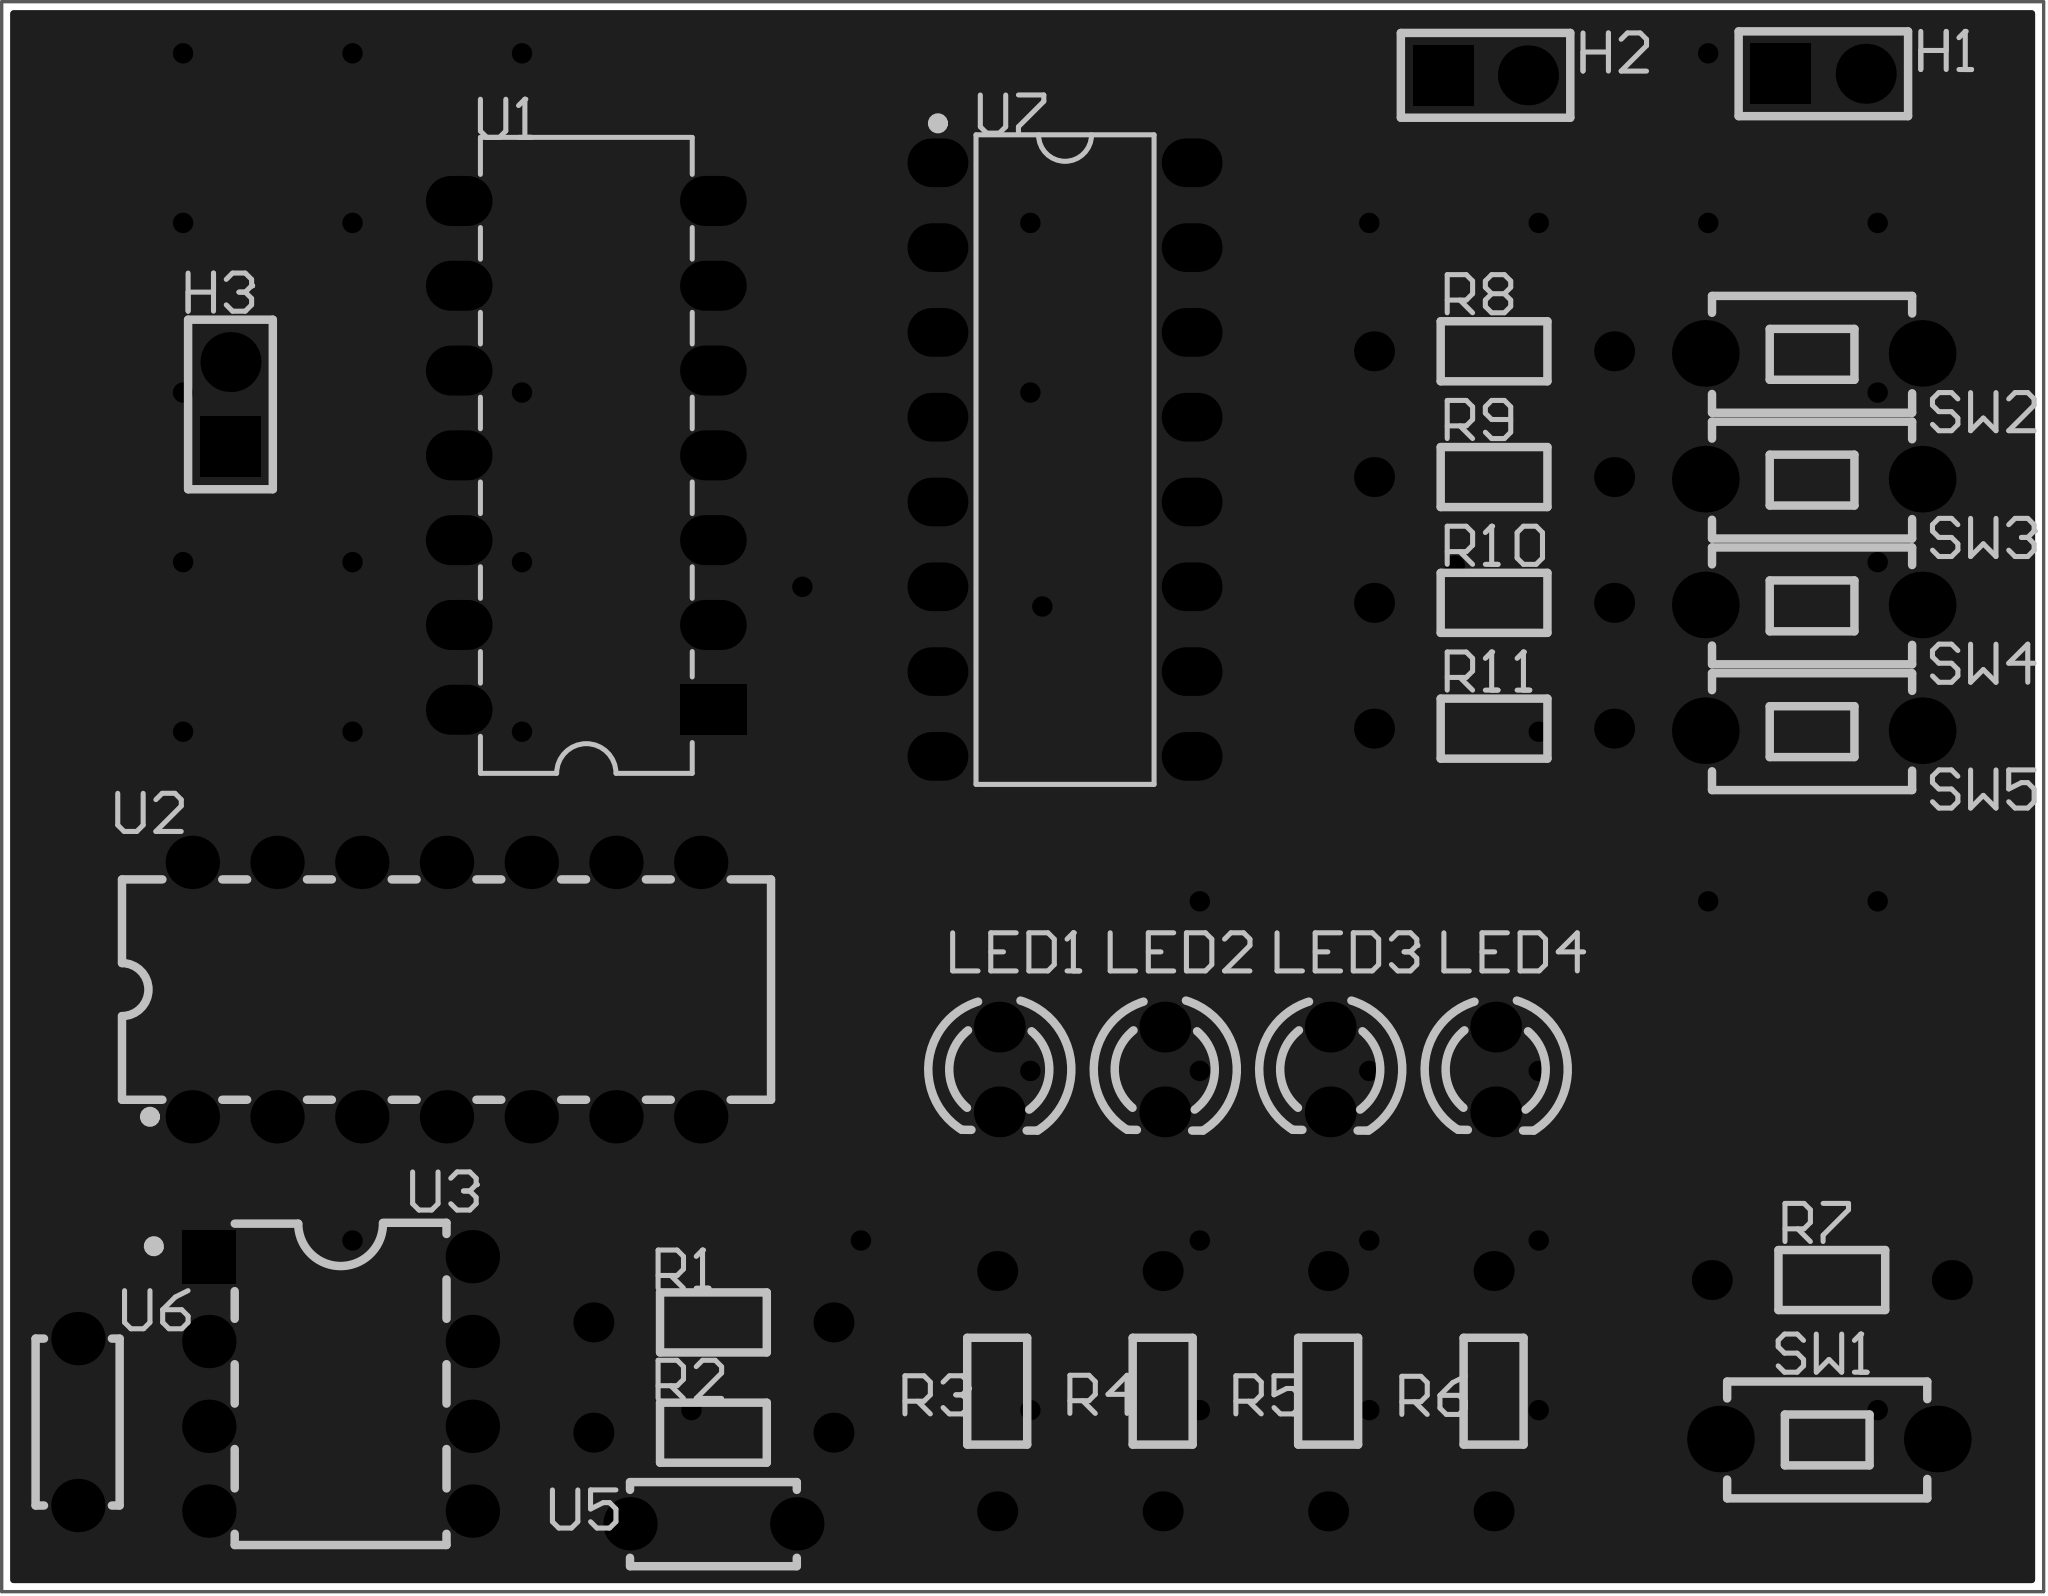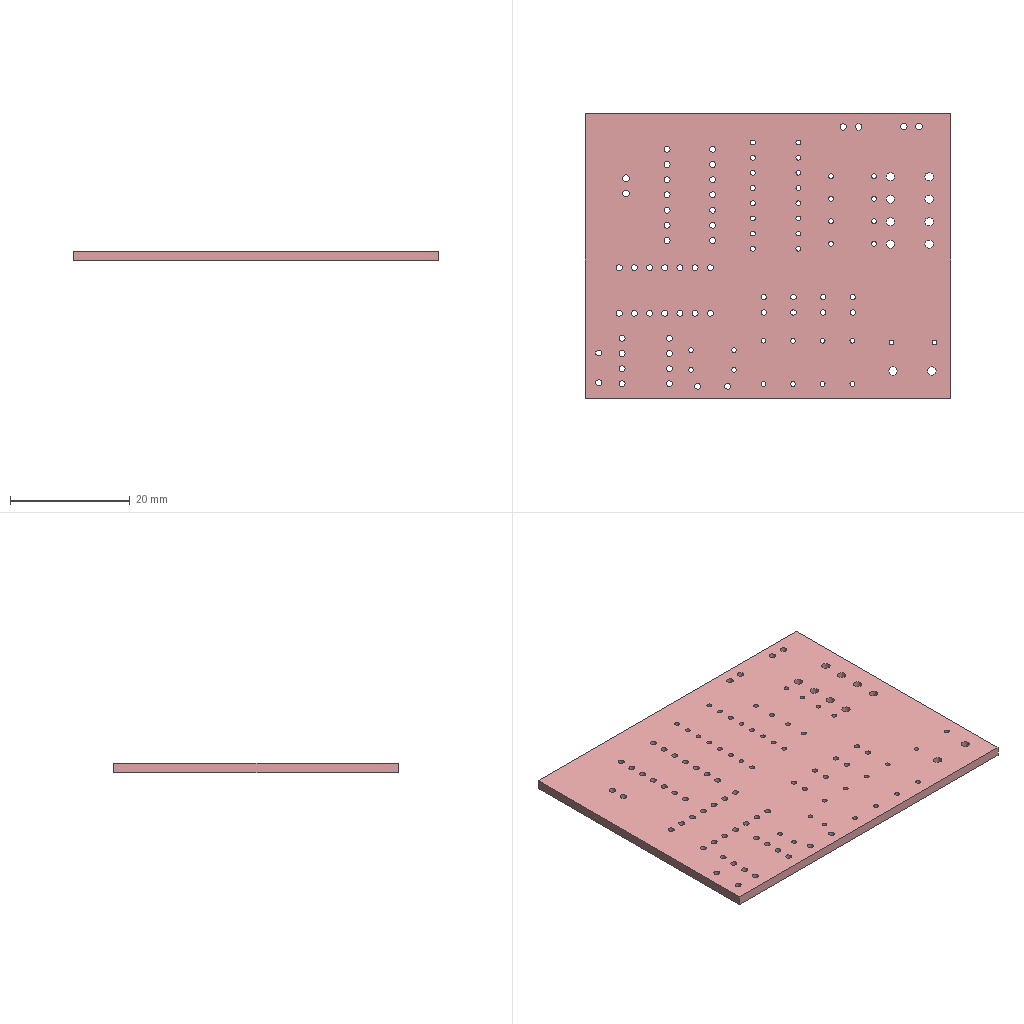Circuit board layout | Altium Designer | box 61.2 x 47.6 x 1.6 mm
Layer stack:
# Altium Designer layer stack of  (unit mm; dielectric type: 0 none, 1 core, 2 prepreg, 3 surface material)
index,name,kind,layer,copper_thickness_mm,dielectric_type,dielectric_thickness_mm,dielectric_material,dielectric_constant
0,Top Paste Mask Layer,other,,,,,,
1,Top Silkscreen Layer,other,,,,,,
2,Top Solder Mask Layer,dielectric,,,3,0.01,,3.3
3,Top Layer,copper,Top Layer,0.035,,,,
4,Dielectric1,dielectric,,,3,1.51,FR4,4.5
5,Bottom Layer,copper,Bottom Layer,0.035,,,,
6,Bottom Solder Mask Layer,dielectric,,,3,0.01,,3.3
7,Bottom Silkscreen Layer,other,,,,,,
8,Bottom Paste Mask Layer,other,,,,,,
# drill layer pairs: low layer,high layer
drill_pair,Top Layer,Bottom Layer
Part placement:
Designator,Comment,Layer,Footprint,Center-X(mm),Center-Y(mm),Rotation
H1,,TopLayer,HDR-TH_2P-P2.54-V-M-1,134.239,123.698,0
H2,,TopLayer,HDR-TH_2P-P2.54-V-M-1,124.113,123.651,0
H3,,TopLayer,HDR-TH_2P-P2.54-V-M-1,86.487,113.792,90
LED1,,TopLayer,LED_TH-3mm,109.535,93.873,270
LED2,,TopLayer,LED_TH-3mm,114.496,93.873,270
LED3,,TopLayer,LED_TH-3mm,119.456,93.873,270
LED4,,TopLayer,LED_TH-3mm,124.416,93.873,270
R1,4.3kΩ,TopLayer,Res_1/8W,100.965,86.296,0
R2,5.1kΩ,TopLayer,Res_1/8W,100.965,82.994,0
R3,220Ω,TopLayer,Res_1/8W,109.473,84.237,90
R4,220Ω,TopLayer,Res_1/8W,114.433,84.237,90
R5,220Ω,TopLayer,Res_1/8W,119.393,84.237,90
R6,220Ω,TopLayer,Res_1/8W,124.353,84.237,90
R7,10kΩ,TopLayer,Res_1/8W,134.493,87.566,0
R8,10kΩ,TopLayer,Res_1/8W,124.367,115.385,0
R9,10kΩ,TopLayer,Res_1/8W,124.367,111.618,0
R10,10kΩ,TopLayer,Res_1/8W,124.367,107.85,0
R11,10kΩ,TopLayer,Res_1/8W,124.367,104.082,0
SW1,,TopLayer,Key_TH_3.5x6x4.3,134.404,82.804,0
SW2,,TopLayer,Key_TH_3.5x6x4.3,133.95,115.322,0
SW3,,TopLayer,Key_TH_3.5x6x4.3,133.95,111.555,0
SW4,,TopLayer,Key_TH_3.5x6x4.3,133.95,107.787,0
SW5,,TopLayer,Key_TH_3.5x6x4.3,133.95,104.02,0
U1,SN74LS20N(XBLW),TopLayer,DIP-14_L19.0-W6.4-P2.54-LS7.6-BL,97.155,112.268,90
U2,SN74LS00NE4,TopLayer,PDIP-14_L19.3-W6.4-P2.54-LS7.9-BL,92.964,96.266,0
U3,LM555CM,TopLayer,PDIP-8_L9.6-W6.4-P2.54-LS7.9-BL-1,89.789,84.455,270
U5,10nF,TopLayer,CAP-TH_L5.0-W2.5-P5.00-D1.0,100.965,80.264,0
U6,100nF,TopLayer,CAP-TH_L5.0-W2.5-P5.00-D1.0,81.915,83.312,270
U7,SN74LS175N,TopLayer,DIP-16_L19.3-W6.4-P2.54-LS7.6-BL,111.506,112.141,270
Pad and via stacks:
# Altium Designer via and pad stacks of  (unit mm). Each distinct definition once, with the count of objects using it.
# via: kind,start_layer,end_layer,hole_mm,diameter_mm,mode(0 simple;1 top-mid-bottom;2 full stack),diameter_per_layer,count,example_net
# pad: kind,layer,hole_mm,hole_type(0 round;1 square;2 slot),plating,top_size,top_shape(1 round;2 rect;3 octagon;9 rounded rect),mid_size,bottom_size,mode,footprint,size_per_layer,count,example
pad,Multi-Layer,1.1,0,plated,1.8x1.8,1,1.8x1.8,1.8x1.8,0,HDR-TH_2P-P2.54-V-M-1,,3,H1.2
pad,Multi-Layer,1.1,0,plated,1.8x1.8,2,1.8x1.8,1.8x1.8,0,HDR-TH_2P-P2.54-V-M-1,,3,H1.1
pad,Multi-Layer,0.9144,0,plated,1.524x1.524,1,1.524x1.524,1.524x1.524,0,LED_TH-3mm,,8,LED1.1
pad,Multi-Layer,0.8001,0,plated,1.199x1.199,1,1.199x1.199,1.199x1.199,0,Res_1/8W,,22,R1.1
pad,Multi-Layer,1.399,0,plated,1.999x1.999,1,1.999x1.999,1.999x1.999,0,Key_TH_3.5x6x4.3,,10,SW1.A
pad,Multi-Layer,1,0,plated,1.5x2,1,1.5x2,1.5x2,0,DIP-14_L19.0-W6.4-P2.54-LS7.6-BL,,13,U1.8
pad,Multi-Layer,1,0,plated,1.5x2,2,1.5x2,1.5x2,0,DIP-14_L19.0-W6.4-P2.54-LS7.6-BL,,1,U1.1
pad,Multi-Layer,1,0,plated,1.6x1.6,1,1.6x1.6,1.6x1.6,0,PDIP-14_L19.3-W6.4-P2.54-LS7.9-BL,,14,U2.9
pad,Multi-Layer,1,0,plated,1.6x1.6,1,1.6x1.6,1.6x1.6,0,PDIP-8_L9.6-W6.4-P2.54-LS7.9-BL-1,,7,U3.8
pad,Multi-Layer,1,0,plated,1.6x1.6,2,1.6x1.6,1.6x1.6,0,PDIP-8_L9.6-W6.4-P2.54-LS7.9-BL-1,,1,U3.1
pad,Multi-Layer,1,0,plated,1.6x1.6,1,1.6x1.6,1.6x1.6,0,CAP-TH_L5.0-W2.5-P5.00-D1.0,,4,U5.1
pad,Multi-Layer,0.8,0,plated,1.46x1.825,1,1.46x1.825,1.46x1.825,0,DIP-16_L19.3-W6.4-P2.54-LS7.6-BL,,16,U7.9
via,Top Layer,Bottom Layer,0.3048,0.61,0,,44,$1N16
Copper pours:
name,layer,net,type(0 solid;1 hatched;2 none)
Top Layer-GND,Top Layer,GND,0
Bottom Layer-GND,Bottom Layer,GND,0
Design rules, without the lines most boards share:
# Altium Designer design rules of  (exported by Altium Designer, unit mm)
# columns: name | kind | enabled | priority | scope1 | scope2 | descriptor | typed fields (field=value)
creepage | 65 | enabled | 1 | All | All | Creepage Distance Constraint =(0mil) (All),(All) |
copperThickness1oz_2 | 2 | enabled | 2 | All | All | Width Constraint (Min=30mil) (Max=100mil) (Preferred=30mil) (All) |